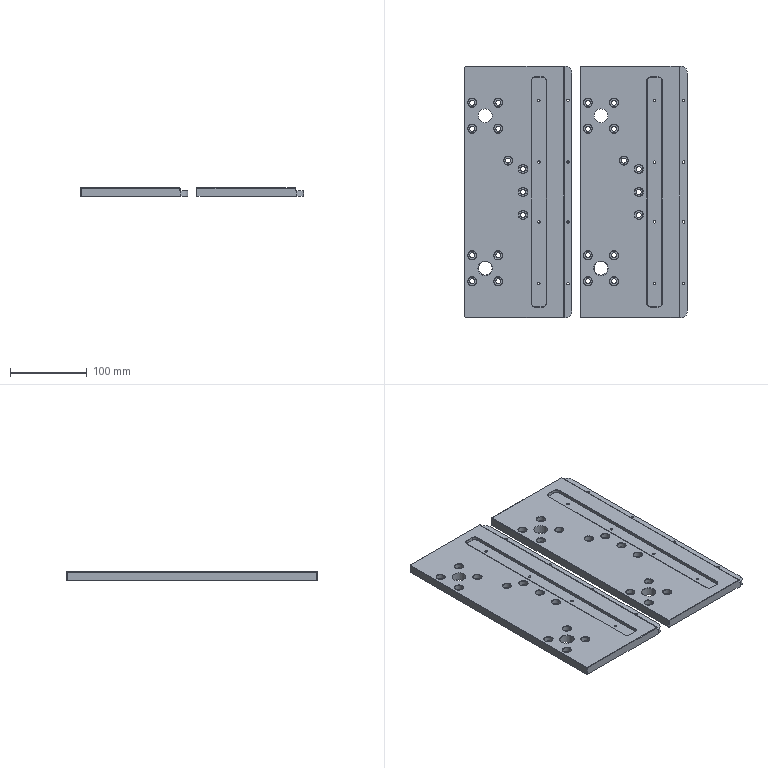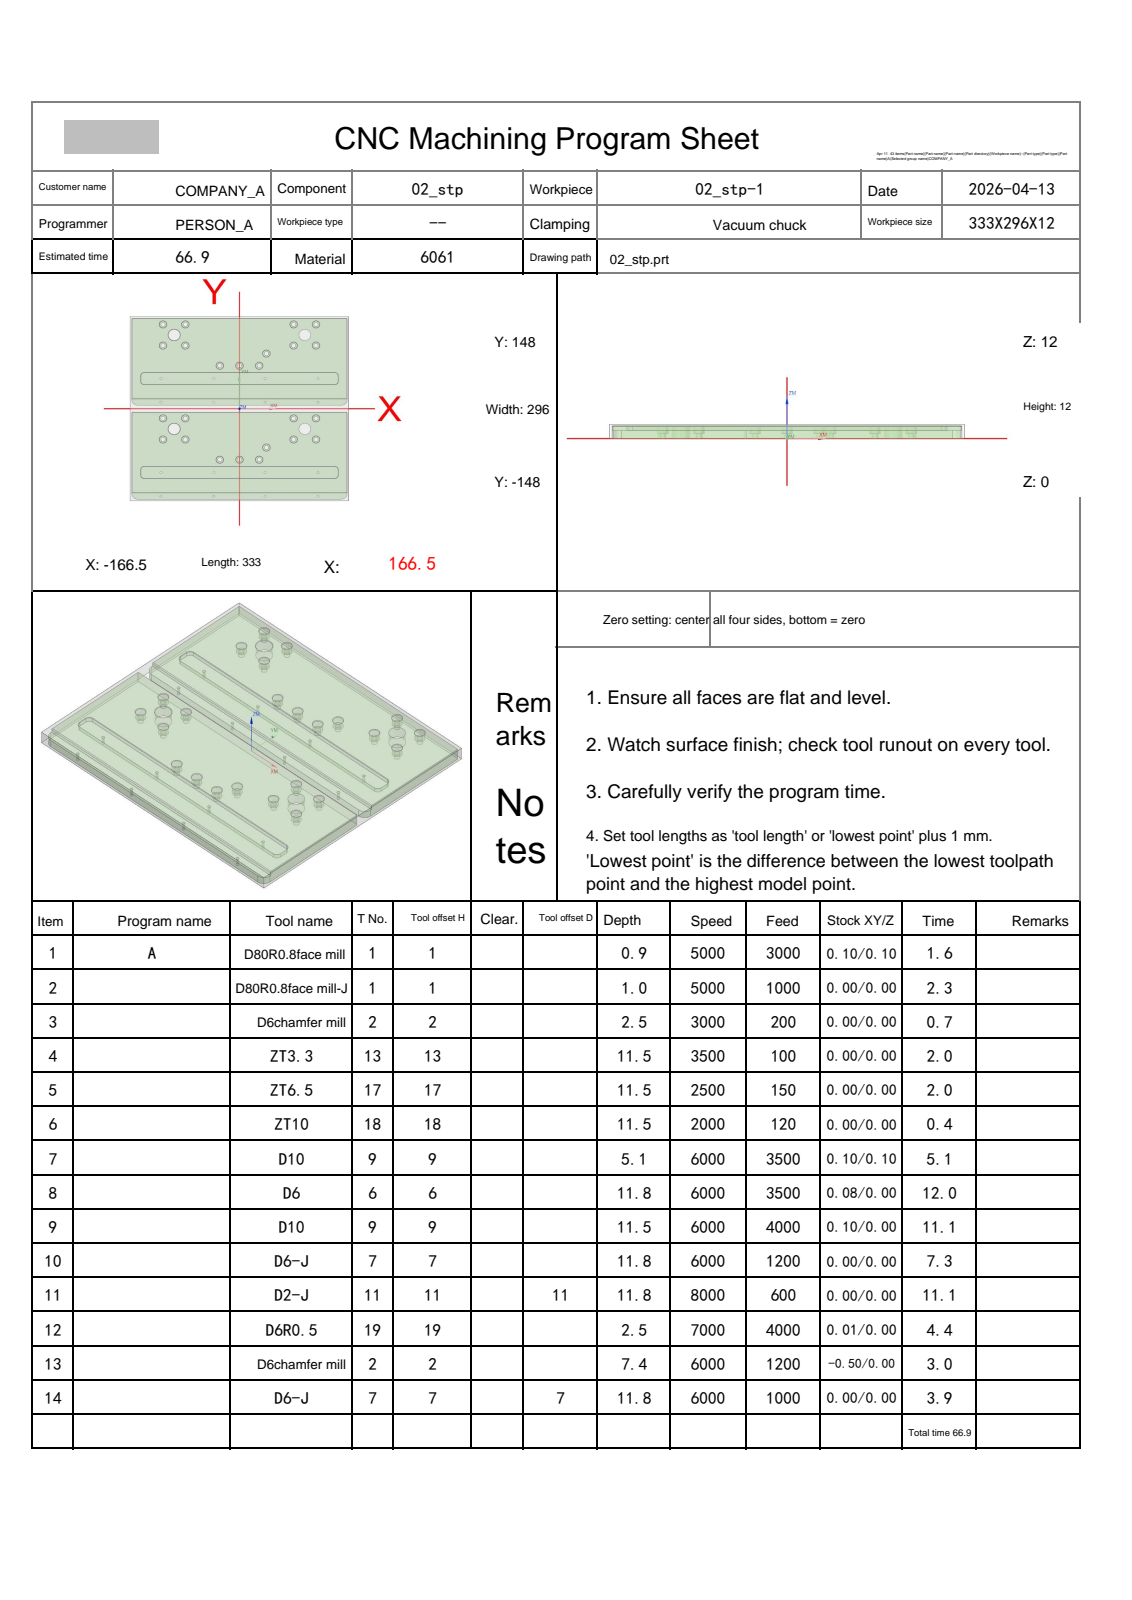NC program | NX | posted by the shop | part box 291 x 328 x 11 mm
Lines 2700 to 3919 of 9762:
N9 T09 M06
(D10  D=10. R=0. H=09 ce=0.10 di=0.00)
G00 G90 G54 X0.0 Y-.4 M03 S6000
G43 H09 Z31.
M08
Z11.5
G01 X163. Z11.415 F4000.
G02 X166.606 Y-1.894 Z11.413 I0.0 J-5.1
G01 X167.606 Y-2.894 Z11.412
G02 X169.1 Y-6.5 Z11.41 I-3.606 J-3.606
G01 Y-136.5 Z11.342
G02 X155. Y-150.6 Z11.331 I-14.1 J0.0
G01 X-155. Z11.169
G02 X-169.1 Y-136.5 Z11.158 I0.0 J14.1
G01 Y-6.5 Z11.09
G02 X-167.606 Y-2.894 Z11.088 I5.1 J0.0
G01 X-166.606 Y-1.894 Z11.087
G02 X-163. Y-.4 Z11.085 I3.606 J-3.606
G01 X163. Z10.915
G02 X166.606 Y-1.894 Z10.913 I0.0 J-5.1
G01 X167.606 Y-2.894 Z10.912
G02 X169.1 Y-6.5 Z10.91 I-3.606 J-3.606
G01 Y-136.5 Z10.842
G02 X155. Y-150.6 Z10.831 I-14.1 J0.0
G01 X-155. Z10.669
G02 X-169.1 Y-136.5 Z10.658 I0.0 J14.1
G01 Y-6.5 Z10.59
G02 X-167.606 Y-2.894 Z10.588 I5.1 J0.0
G01 X-166.606 Y-1.894 Z10.587
G02 X-163. Y-.4 Z10.585 I3.606 J-3.606
G01 X163. Z10.415
G02 X166.606 Y-1.894 Z10.413 I0.0 J-5.1
G01 X167.606 Y-2.894 Z10.412
G02 X169.1 Y-6.5 Z10.41 I-3.606 J-3.606
G01 Y-136.5 Z10.342
G02 X155. Y-150.6 Z10.331 I-14.1 J0.0
G01 X-155. Z10.169
G02 X-169.1 Y-136.5 Z10.158 I0.0 J14.1
G01 Y-6.5 Z10.09
G02 X-167.606 Y-2.894 Z10.088 I5.1 J0.0
G01 X-166.606 Y-1.894 Z10.087
G02 X-163. Y-.4 Z10.085 I3.606 J-3.606
G01 X163. Z9.915
G02 X166.606 Y-1.894 Z9.913 I0.0 J-5.1
G01 X167.606 Y-2.894 Z9.912
G02 X169.1 Y-6.5 Z9.91 I-3.606 J-3.606
G01 Y-136.5 Z9.842
G02 X155. Y-150.6 Z9.831 I-14.1 J0.0
G01 X-155. Z9.669
G02 X-169.1 Y-136.5 Z9.658 I0.0 J14.1
G01 Y-6.5 Z9.59
G02 X-167.606 Y-2.894 Z9.588 I5.1 J0.0
G01 X-166.606 Y-1.894 Z9.587
G02 X-163. Y-.4 Z9.585 I3.606 J-3.606
G01 X163. Z9.415
G02 X166.606 Y-1.894 Z9.413 I0.0 J-5.1
G01 X167.606 Y-2.894 Z9.412
G02 X169.1 Y-6.5 Z9.41 I-3.606 J-3.606
G01 Y-136.5 Z9.342
G02 X155. Y-150.6 Z9.331 I-14.1 J0.0
G01 X-155. Z9.169
G02 X-169.1 Y-136.5 Z9.158 I0.0 J14.1
G01 Y-6.5 Z9.09
G02 X-167.606 Y-2.894 Z9.088 I5.1 J0.0
G01 X-166.606 Y-1.894 Z9.087
G02 X-163. Y-.4 Z9.085 I3.606 J-3.606
G01 X163. Z8.915
G02 X166.606 Y-1.894 Z8.913 I0.0 J-5.1
G01 X167.606 Y-2.894 Z8.912
G02 X169.1 Y-6.5 Z8.91 I-3.606 J-3.606
G01 Y-136.5 Z8.842
G02 X155. Y-150.6 Z8.831 I-14.1 J0.0
G01 X-155. Z8.669
G02 X-169.1 Y-136.5 Z8.658 I0.0 J14.1
G01 Y-6.5 Z8.59
G02 X-167.606 Y-2.894 Z8.588 I5.1 J0.0
G01 X-166.606 Y-1.894 Z8.587
G02 X-163. Y-.4 Z8.585 I3.606 J-3.606
G01 X163. Z8.415
G02 X166.606 Y-1.894 Z8.413 I0.0 J-5.1
G01 X167.606 Y-2.894 Z8.412
G02 X169.1 Y-6.5 Z8.41 I-3.606 J-3.606
G01 Y-136.5 Z8.342
G02 X155. Y-150.6 Z8.331 I-14.1 J0.0
G01 X-155. Z8.169
G02 X-169.1 Y-136.5 Z8.158 I0.0 J14.1
G01 Y-6.5 Z8.09
G02 X-167.606 Y-2.894 Z8.088 I5.1 J0.0
G01 X-166.606 Y-1.894 Z8.087
G02 X-163. Y-.4 Z8.085 I3.606 J-3.606
G01 X163. Z7.915
G02 X166.606 Y-1.894 Z7.913 I0.0 J-5.1
G01 X167.606 Y-2.894 Z7.912
G02 X169.1 Y-6.5 Z7.91 I-3.606 J-3.606
G01 Y-136.5 Z7.842
G02 X155. Y-150.6 Z7.831 I-14.1 J0.0
G01 X-155. Z7.669
G02 X-169.1 Y-136.5 Z7.658 I0.0 J14.1
G01 Y-6.5 Z7.59
G02 X-167.606 Y-2.894 Z7.588 I5.1 J0.0
G01 X-166.606 Y-1.894 Z7.587
G02 X-163. Y-.4 Z7.585 I3.606 J-3.606
G01 X163. Z7.415
G02 X166.606 Y-1.894 Z7.413 I0.0 J-5.1
G01 X167.606 Y-2.894 Z7.412
G02 X169.1 Y-6.5 Z7.41 I-3.606 J-3.606
G01 Y-136.5 Z7.342
G02 X155. Y-150.6 Z7.331 I-14.1 J0.0
G01 X-155. Z7.169
G02 X-169.1 Y-136.5 Z7.158 I0.0 J14.1
G01 Y-6.5 Z7.09
G02 X-167.606 Y-2.894 Z7.088 I5.1 J0.0
G01 X-166.606 Y-1.894 Z7.087
G02 X-163. Y-.4 Z7.085 I3.606 J-3.606
G01 X163. Z6.915
G02 X166.606 Y-1.894 Z6.913 I0.0 J-5.1
G01 X167.606 Y-2.894 Z6.912
G02 X169.1 Y-6.5 Z6.91 I-3.606 J-3.606
G01 Y-136.5 Z6.842
G02 X155. Y-150.6 Z6.831 I-14.1 J0.0
G01 X-155. Z6.669
G02 X-169.1 Y-136.5 Z6.658 I0.0 J14.1
G01 Y-6.5 Z6.59
G02 X-167.606 Y-2.894 Z6.588 I5.1 J0.0
G01 X-166.606 Y-1.894 Z6.587
G02 X-163. Y-.4 Z6.585 I3.606 J-3.606
G01 X163. Z6.415
G02 X166.606 Y-1.894 Z6.413 I0.0 J-5.1
G01 X167.606 Y-2.894 Z6.412
G02 X169.1 Y-6.5 Z6.41 I-3.606 J-3.606
G01 Y-136.5 Z6.342
G02 X155. Y-150.6 Z6.331 I-14.1 J0.0
G01 X-155. Z6.169
G02 X-169.1 Y-136.5 Z6.158 I0.0 J14.1
G01 Y-6.5 Z6.09
G02 X-167.606 Y-2.894 Z6.088 I5.1 J0.0
G01 X-166.606 Y-1.894 Z6.087
G02 X-163. Y-.4 Z6.085 I3.606 J-3.606
G01 X163. Z5.915
G02 X166.606 Y-1.894 Z5.913 I0.0 J-5.1
G01 X167.606 Y-2.894 Z5.912
G02 X169.1 Y-6.5 Z5.91 I-3.606 J-3.606
G01 Y-136.5 Z5.842
G02 X155. Y-150.6 Z5.831 I-14.1 J0.0
G01 X-155. Z5.669
G02 X-169.1 Y-136.5 Z5.658 I0.0 J14.1
G01 Y-6.5 Z5.59
G02 X-167.606 Y-2.894 Z5.588 I5.1 J0.0
G01 X-166.606 Y-1.894 Z5.587
G02 X-163. Y-.4 Z5.585 I3.606 J-3.606
G01 X163. Z5.415
G02 X166.606 Y-1.894 Z5.413 I0.0 J-5.1
G01 X167.606 Y-2.894 Z5.412
G02 X169.1 Y-6.5 Z5.41 I-3.606 J-3.606
G01 Y-136.5 Z5.342
G02 X155. Y-150.6 Z5.331 I-14.1 J0.0
G01 X-155. Z5.169
G02 X-169.1 Y-136.5 Z5.158 I0.0 J14.1
G01 Y-6.5 Z5.09
G02 X-167.606 Y-2.894 Z5.088 I5.1 J0.0
G01 X-166.606 Y-1.894 Z5.087
G02 X-163. Y-.4 Z5.085 I3.606 J-3.606
G01 X163. Z4.915
G02 X166.606 Y-1.894 Z4.913 I0.0 J-5.1
G01 X167.606 Y-2.894 Z4.912
G02 X169.1 Y-6.5 Z4.91 I-3.606 J-3.606
G01 Y-136.5 Z4.842
G02 X155. Y-150.6 Z4.831 I-14.1 J0.0
G01 X-155. Z4.669
G02 X-169.1 Y-136.5 Z4.658 I0.0 J14.1
G01 Y-6.5 Z4.59
G02 X-167.606 Y-2.894 Z4.588 I5.1 J0.0
G01 X-166.606 Y-1.894 Z4.587
G02 X-163. Y-.4 Z4.585 I3.606 J-3.606
G01 X163. Z4.415
G02 X166.606 Y-1.894 Z4.413 I0.0 J-5.1
G01 X167.606 Y-2.894 Z4.412
G02 X169.1 Y-6.5 Z4.41 I-3.606 J-3.606
G01 Y-136.5 Z4.342
G02 X155. Y-150.6 Z4.331 I-14.1 J0.0
G01 X-155. Z4.169
G02 X-169.1 Y-136.5 Z4.158 I0.0 J14.1
G01 Y-6.5 Z4.09
G02 X-167.606 Y-2.894 Z4.088 I5.1 J0.0
G01 X-166.606 Y-1.894 Z4.087
G02 X-163. Y-.4 Z4.085 I3.606 J-3.606
G01 X163. Z3.915
G02 X166.606 Y-1.894 Z3.913 I0.0 J-5.1
G01 X167.606 Y-2.894 Z3.912
G02 X169.1 Y-6.5 Z3.91 I-3.606 J-3.606
G01 Y-136.5 Z3.842
G02 X155. Y-150.6 Z3.831 I-14.1 J0.0
G01 X-155. Z3.669
G02 X-169.1 Y-136.5 Z3.658 I0.0 J14.1
G01 Y-6.5 Z3.59
G02 X-167.606 Y-2.894 Z3.588 I5.1 J0.0
G01 X-166.606 Y-1.894 Z3.587
G02 X-163. Y-.4 Z3.585 I3.606 J-3.606
G01 X163. Z3.415
G02 X166.606 Y-1.894 Z3.413 I0.0 J-5.1
G01 X167.606 Y-2.894 Z3.412
G02 X169.1 Y-6.5 Z3.41 I-3.606 J-3.606
G01 Y-136.5 Z3.342
G02 X155. Y-150.6 Z3.331 I-14.1 J0.0
G01 X-155. Z3.169
G02 X-169.1 Y-136.5 Z3.158 I0.0 J14.1
G01 Y-6.5 Z3.09
G02 X-167.606 Y-2.894 Z3.088 I5.1 J0.0
G01 X-166.606 Y-1.894 Z3.087
G02 X-163. Y-.4 Z3.085 I3.606 J-3.606
G01 X163. Z2.915
G02 X166.606 Y-1.894 Z2.913 I0.0 J-5.1
G01 X167.606 Y-2.894 Z2.912
G02 X169.1 Y-6.5 Z2.91 I-3.606 J-3.606
G01 Y-136.5 Z2.842
G02 X155. Y-150.6 Z2.831 I-14.1 J0.0
G01 X-155. Z2.669
G02 X-169.1 Y-136.5 Z2.658 I0.0 J14.1
G01 Y-6.5 Z2.59
G02 X-167.606 Y-2.894 Z2.588 I5.1 J0.0
G01 X-166.606 Y-1.894 Z2.587
G02 X-163. Y-.4 Z2.585 I3.606 J-3.606
G01 X163. Z2.415
G02 X166.606 Y-1.894 Z2.413 I0.0 J-5.1
G01 X167.606 Y-2.894 Z2.412
G02 X169.1 Y-6.5 Z2.41 I-3.606 J-3.606
G01 Y-136.5 Z2.342
G02 X155. Y-150.6 Z2.331 I-14.1 J0.0
G01 X-155. Z2.169
G02 X-169.1 Y-136.5 Z2.158 I0.0 J14.1
G01 Y-6.5 Z2.09
G02 X-167.606 Y-2.894 Z2.088 I5.1 J0.0
G01 X-166.606 Y-1.894 Z2.087
G02 X-163. Y-.4 Z2.085 I3.606 J-3.606
G01 X163. Z1.915
G02 X166.606 Y-1.894 Z1.913 I0.0 J-5.1
G01 X167.606 Y-2.894 Z1.912
G02 X169.1 Y-6.5 Z1.91 I-3.606 J-3.606
G01 Y-136.5 Z1.842
G02 X155. Y-150.6 Z1.831 I-14.1 J0.0
G01 X-155. Z1.669
G02 X-169.1 Y-136.5 Z1.658 I0.0 J14.1
G01 Y-6.5 Z1.59
G02 X-167.606 Y-2.894 Z1.588 I5.1 J0.0
G01 X-166.606 Y-1.894 Z1.587
G02 X-163. Y-.4 Z1.585 I3.606 J-3.606
G01 X163. Z1.415
G02 X166.606 Y-1.894 Z1.413 I0.0 J-5.1
G01 X167.606 Y-2.894 Z1.412
G02 X169.1 Y-6.5 Z1.41 I-3.606 J-3.606
G01 Y-136.5 Z1.342
G02 X155. Y-150.6 Z1.331 I-14.1 J0.0
G01 X-155. Z1.169
G02 X-169.1 Y-136.5 Z1.158 I0.0 J14.1
G01 Y-6.5 Z1.09
G02 X-167.606 Y-2.894 Z1.088 I5.1 J0.0
G01 X-166.606 Y-1.894 Z1.087
G02 X-163. Y-.4 Z1.085 I3.606 J-3.606
G01 X163. Z.915
G02 X166.606 Y-1.894 Z.913 I0.0 J-5.1
G01 X167.606 Y-2.894 Z.912
G02 X169.1 Y-6.5 Z.91 I-3.606 J-3.606
G01 Y-136.5 Z.842
G02 X155. Y-150.6 Z.831 I-14.1 J0.0
G01 X-155. Z.669
G02 X-169.1 Y-136.5 Z.658 I0.0 J14.1
G01 Y-6.5 Z.59
G02 X-167.606 Y-2.894 Z.588 I5.1 J0.0
G01 X-166.606 Y-1.894 Z.587
G02 X-163. Y-.4 Z.585 I3.606 J-3.606
G01 X0.0 Z.5
X163.
G02 X166.606 Y-1.894 I0.0 J-5.1
G01 X167.606 Y-2.894
G02 X169.1 Y-6.5 I-3.606 J-3.606
G01 Y-136.5
G02 X155. Y-150.6 I-14.1 J0.0
G01 X-155.
G02 X-169.1 Y-136.5 I0.0 J14.1
G01 Y-6.5
G02 X-167.606 Y-2.894 I5.1 J0.0
G01 X-166.606 Y-1.894
G02 X-163. Y-.4 I3.606 J-3.606
G01 X0.0
X.5
Z1.5
G00 Z31.
X0.0 Y150.6
Z11.5
G01 X163. Z11.415
G02 X166.606 Y149.106 Z11.413 I0.0 J-5.1
G01 X167.606 Y148.106 Z11.412
G02 X169.1 Y144.5 Z11.41 I-3.606 J-3.606
G01 Y14.5 Z11.342
G02 X155. Y.4 Z11.331 I-14.1 J0.0
G01 X-155. Z11.169
G02 X-169.1 Y14.5 Z11.158 I0.0 J14.1
G01 Y144.5 Z11.09
G02 X-167.606 Y148.106 Z11.088 I5.1 J0.0
G01 X-166.606 Y149.106 Z11.087
G02 X-163. Y150.6 Z11.085 I3.606 J-3.606
G01 X163. Z10.915
G02 X166.606 Y149.106 Z10.913 I0.0 J-5.1
G01 X167.606 Y148.106 Z10.912
G02 X169.1 Y144.5 Z10.91 I-3.606 J-3.606
G01 Y14.5 Z10.842
G02 X155. Y.4 Z10.831 I-14.1 J0.0
G01 X-155. Z10.669
G02 X-169.1 Y14.5 Z10.658 I0.0 J14.1
G01 Y144.5 Z10.59
G02 X-167.606 Y148.106 Z10.588 I5.1 J0.0
G01 X-166.606 Y149.106 Z10.587
G02 X-163. Y150.6 Z10.585 I3.606 J-3.606
G01 X163. Z10.415
G02 X166.606 Y149.106 Z10.413 I0.0 J-5.1
G01 X167.606 Y148.106 Z10.412
G02 X169.1 Y144.5 Z10.41 I-3.606 J-3.606
G01 Y14.5 Z10.342
G02 X155. Y.4 Z10.331 I-14.1 J0.0
G01 X-155. Z10.169
G02 X-169.1 Y14.5 Z10.158 I0.0 J14.1
G01 Y144.5 Z10.09
G02 X-167.606 Y148.106 Z10.088 I5.1 J0.0
G01 X-166.606 Y149.106 Z10.087
G02 X-163. Y150.6 Z10.085 I3.606 J-3.606
G01 X163. Z9.915
G02 X166.606 Y149.106 Z9.913 I0.0 J-5.1
G01 X167.606 Y148.106 Z9.912
G02 X169.1 Y144.5 Z9.91 I-3.606 J-3.606
G01 Y14.5 Z9.842
G02 X155. Y.4 Z9.831 I-14.1 J0.0
G01 X-155. Z9.669
G02 X-169.1 Y14.5 Z9.658 I0.0 J14.1
G01 Y144.5 Z9.59
G02 X-167.606 Y148.106 Z9.588 I5.1 J0.0
G01 X-166.606 Y149.106 Z9.587
G02 X-163. Y150.6 Z9.585 I3.606 J-3.606
G01 X163. Z9.415
G02 X166.606 Y149.106 Z9.413 I0.0 J-5.1
G01 X167.606 Y148.106 Z9.412
G02 X169.1 Y144.5 Z9.41 I-3.606 J-3.606
G01 Y14.5 Z9.342
G02 X155. Y.4 Z9.331 I-14.1 J0.0
G01 X-155. Z9.169
G02 X-169.1 Y14.5 Z9.158 I0.0 J14.1
G01 Y144.5 Z9.09
G02 X-167.606 Y148.106 Z9.088 I5.1 J0.0
G01 X-166.606 Y149.106 Z9.087
G02 X-163. Y150.6 Z9.085 I3.606 J-3.606
G01 X163. Z8.915
G02 X166.606 Y149.106 Z8.913 I0.0 J-5.1
G01 X167.606 Y148.106 Z8.912
G02 X169.1 Y144.5 Z8.91 I-3.606 J-3.606
G01 Y14.5 Z8.842
G02 X155. Y.4 Z8.831 I-14.1 J0.0
G01 X-155. Z8.669
G02 X-169.1 Y14.5 Z8.658 I0.0 J14.1
G01 Y144.5 Z8.59
G02 X-167.606 Y148.106 Z8.588 I5.1 J0.0
G01 X-166.606 Y149.106 Z8.587
G02 X-163. Y150.6 Z8.585 I3.606 J-3.606
G01 X163. Z8.415
G02 X166.606 Y149.106 Z8.413 I0.0 J-5.1
G01 X167.606 Y148.106 Z8.412
G02 X169.1 Y144.5 Z8.41 I-3.606 J-3.606
G01 Y14.5 Z8.342
G02 X155. Y.4 Z8.331 I-14.1 J0.0
G01 X-155. Z8.169
G02 X-169.1 Y14.5 Z8.158 I0.0 J14.1
G01 Y144.5 Z8.09
G02 X-167.606 Y148.106 Z8.088 I5.1 J0.0
G01 X-166.606 Y149.106 Z8.087
G02 X-163. Y150.6 Z8.085 I3.606 J-3.606
G01 X163. Z7.915
G02 X166.606 Y149.106 Z7.913 I0.0 J-5.1
G01 X167.606 Y148.106 Z7.912
G02 X169.1 Y144.5 Z7.91 I-3.606 J-3.606
G01 Y14.5 Z7.842
G02 X155. Y.4 Z7.831 I-14.1 J0.0
G01 X-155. Z7.669
G02 X-169.1 Y14.5 Z7.658 I0.0 J14.1
G01 Y144.5 Z7.59
G02 X-167.606 Y148.106 Z7.588 I5.1 J0.0
G01 X-166.606 Y149.106 Z7.587
G02 X-163. Y150.6 Z7.585 I3.606 J-3.606
G01 X163. Z7.415
G02 X166.606 Y149.106 Z7.413 I0.0 J-5.1
G01 X167.606 Y148.106 Z7.412
G02 X169.1 Y144.5 Z7.41 I-3.606 J-3.606
G01 Y14.5 Z7.342
G02 X155. Y.4 Z7.331 I-14.1 J0.0
G01 X-155. Z7.169
G02 X-169.1 Y14.5 Z7.158 I0.0 J14.1
G01 Y144.5 Z7.09
G02 X-167.606 Y148.106 Z7.088 I5.1 J0.0
G01 X-166.606 Y149.106 Z7.087
G02 X-163. Y150.6 Z7.085 I3.606 J-3.606
G01 X163. Z6.915
G02 X166.606 Y149.106 Z6.913 I0.0 J-5.1
G01 X167.606 Y148.106 Z6.912
G02 X169.1 Y144.5 Z6.91 I-3.606 J-3.606
G01 Y14.5 Z6.842
G02 X155. Y.4 Z6.831 I-14.1 J0.0
G01 X-155. Z6.669
G02 X-169.1 Y14.5 Z6.658 I0.0 J14.1
G01 Y144.5 Z6.59
G02 X-167.606 Y148.106 Z6.588 I5.1 J0.0
G01 X-166.606 Y149.106 Z6.587
G02 X-163. Y150.6 Z6.585 I3.606 J-3.606
G01 X163. Z6.415
G02 X166.606 Y149.106 Z6.413 I0.0 J-5.1
G01 X167.606 Y148.106 Z6.412
G02 X169.1 Y144.5 Z6.41 I-3.606 J-3.606
G01 Y14.5 Z6.342
G02 X155. Y.4 Z6.331 I-14.1 J0.0
G01 X-155. Z6.169
G02 X-169.1 Y14.5 Z6.158 I0.0 J14.1
G01 Y144.5 Z6.09
G02 X-167.606 Y148.106 Z6.088 I5.1 J0.0
G01 X-166.606 Y149.106 Z6.087
G02 X-163. Y150.6 Z6.085 I3.606 J-3.606
G01 X163. Z5.915
G02 X166.606 Y149.106 Z5.913 I0.0 J-5.1
G01 X167.606 Y148.106 Z5.912
G02 X169.1 Y144.5 Z5.91 I-3.606 J-3.606
G01 Y14.5 Z5.842
G02 X155. Y.4 Z5.831 I-14.1 J0.0
G01 X-155. Z5.669
G02 X-169.1 Y14.5 Z5.658 I0.0 J14.1
G01 Y144.5 Z5.59
G02 X-167.606 Y148.106 Z5.588 I5.1 J0.0
G01 X-166.606 Y149.106 Z5.587
G02 X-163. Y150.6 Z5.585 I3.606 J-3.606
G01 X163. Z5.415
G02 X166.606 Y149.106 Z5.413 I0.0 J-5.1
G01 X167.606 Y148.106 Z5.412
G02 X169.1 Y144.5 Z5.41 I-3.606 J-3.606
G01 Y14.5 Z5.342
G02 X155. Y.4 Z5.331 I-14.1 J0.0
G01 X-155. Z5.169
G02 X-169.1 Y14.5 Z5.158 I0.0 J14.1
G01 Y144.5 Z5.09
G02 X-167.606 Y148.106 Z5.088 I5.1 J0.0
G01 X-166.606 Y149.106 Z5.087
G02 X-163. Y150.6 Z5.085 I3.606 J-3.606
G01 X163. Z4.915
G02 X166.606 Y149.106 Z4.913 I0.0 J-5.1
G01 X167.606 Y148.106 Z4.912
G02 X169.1 Y144.5 Z4.91 I-3.606 J-3.606
G01 Y14.5 Z4.842
G02 X155. Y.4 Z4.831 I-14.1 J0.0
G01 X-155. Z4.669
G02 X-169.1 Y14.5 Z4.658 I0.0 J14.1
G01 Y144.5 Z4.59
G02 X-167.606 Y148.106 Z4.588 I5.1 J0.0
G01 X-166.606 Y149.106 Z4.587
G02 X-163. Y150.6 Z4.585 I3.606 J-3.606
G01 X163. Z4.415
G02 X166.606 Y149.106 Z4.413 I0.0 J-5.1
G01 X167.606 Y148.106 Z4.412
G02 X169.1 Y144.5 Z4.41 I-3.606 J-3.606
G01 Y14.5 Z4.342
G02 X155. Y.4 Z4.331 I-14.1 J0.0
G01 X-155. Z4.169
G02 X-169.1 Y14.5 Z4.158 I0.0 J14.1
G01 Y144.5 Z4.09
G02 X-167.606 Y148.106 Z4.088 I5.1 J0.0
G01 X-166.606 Y149.106 Z4.087
G02 X-163. Y150.6 Z4.085 I3.606 J-3.606
G01 X163. Z3.915
G02 X166.606 Y149.106 Z3.913 I0.0 J-5.1
G01 X167.606 Y148.106 Z3.912
G02 X169.1 Y144.5 Z3.91 I-3.606 J-3.606
G01 Y14.5 Z3.842
G02 X155. Y.4 Z3.831 I-14.1 J0.0
G01 X-155. Z3.669
G02 X-169.1 Y14.5 Z3.658 I0.0 J14.1
G01 Y144.5 Z3.59
G02 X-167.606 Y148.106 Z3.588 I5.1 J0.0
G01 X-166.606 Y149.106 Z3.587
G02 X-163. Y150.6 Z3.585 I3.606 J-3.606
G01 X163. Z3.415
G02 X166.606 Y149.106 Z3.413 I0.0 J-5.1
G01 X167.606 Y148.106 Z3.412
G02 X169.1 Y144.5 Z3.41 I-3.606 J-3.606
G01 Y14.5 Z3.342
G02 X155. Y.4 Z3.331 I-14.1 J0.0
G01 X-155. Z3.169
G02 X-169.1 Y14.5 Z3.158 I0.0 J14.1
G01 Y144.5 Z3.09
G02 X-167.606 Y148.106 Z3.088 I5.1 J0.0
G01 X-166.606 Y149.106 Z3.087
G02 X-163. Y150.6 Z3.085 I3.606 J-3.606
G01 X163. Z2.915
G02 X166.606 Y149.106 Z2.913 I0.0 J-5.1
G01 X167.606 Y148.106 Z2.912
G02 X169.1 Y144.5 Z2.91 I-3.606 J-3.606
G01 Y14.5 Z2.842
G02 X155. Y.4 Z2.831 I-14.1 J0.0
G01 X-155. Z2.669
G02 X-169.1 Y14.5 Z2.658 I0.0 J14.1
G01 Y144.5 Z2.59
G02 X-167.606 Y148.106 Z2.588 I5.1 J0.0
G01 X-166.606 Y149.106 Z2.587
G02 X-163. Y150.6 Z2.585 I3.606 J-3.606
G01 X163. Z2.415
G02 X166.606 Y149.106 Z2.413 I0.0 J-5.1
G01 X167.606 Y148.106 Z2.412
G02 X169.1 Y144.5 Z2.41 I-3.606 J-3.606
G01 Y14.5 Z2.342
G02 X155. Y.4 Z2.331 I-14.1 J0.0
G01 X-155. Z2.169
G02 X-169.1 Y14.5 Z2.158 I0.0 J14.1
G01 Y144.5 Z2.09
G02 X-167.606 Y148.106 Z2.088 I5.1 J0.0
G01 X-166.606 Y149.106 Z2.087
G02 X-163. Y150.6 Z2.085 I3.606 J-3.606
G01 X163. Z1.915
G02 X166.606 Y149.106 Z1.913 I0.0 J-5.1
G01 X167.606 Y148.106 Z1.912
G02 X169.1 Y144.5 Z1.91 I-3.606 J-3.606
G01 Y14.5 Z1.842
G02 X155. Y.4 Z1.831 I-14.1 J0.0
G01 X-155. Z1.669
G02 X-169.1 Y14.5 Z1.658 I0.0 J14.1
G01 Y144.5 Z1.59
G02 X-167.606 Y148.106 Z1.588 I5.1 J0.0
G01 X-166.606 Y149.106 Z1.587
G02 X-163. Y150.6 Z1.585 I3.606 J-3.606
G01 X163. Z1.415
G02 X166.606 Y149.106 Z1.413 I0.0 J-5.1
G01 X167.606 Y148.106 Z1.412
G02 X169.1 Y144.5 Z1.41 I-3.606 J-3.606
G01 Y14.5 Z1.342
G02 X155. Y.4 Z1.331 I-14.1 J0.0
G01 X-155. Z1.169
G02 X-169.1 Y14.5 Z1.158 I0.0 J14.1
G01 Y144.5 Z1.09
G02 X-167.606 Y148.106 Z1.088 I5.1 J0.0
G01 X-166.606 Y149.106 Z1.087
G02 X-163. Y150.6 Z1.085 I3.606 J-3.606
G01 X163. Z.915
G02 X166.606 Y149.106 Z.913 I0.0 J-5.1
G01 X167.606 Y148.106 Z.912
G02 X169.1 Y144.5 Z.91 I-3.606 J-3.606
G01 Y14.5 Z.842
G02 X155. Y.4 Z.831 I-14.1 J0.0
G01 X-155. Z.669
G02 X-169.1 Y14.5 Z.658 I0.0 J14.1
G01 Y144.5 Z.59
G02 X-167.606 Y148.106 Z.588 I5.1 J0.0
G01 X-166.606 Y149.106 Z.587
G02 X-163. Y150.6 Z.585 I3.606 J-3.606
G01 X0.0 Z.5
X163.
G02 X166.606 Y149.106 I0.0 J-5.1
G01 X167.606 Y148.106
G02 X169.1 Y144.5 I-3.606 J-3.606
G01 Y14.5
G02 X155. Y.4 I-14.1 J0.0
G01 X-155.
G02 X-169.1 Y14.5 I0.0 J14.1
G01 Y144.5
G02 X-167.606 Y148.106 I5.1 J0.0
G01 X-166.606 Y149.106
G02 X-163. Y150.6 I3.606 J-3.606
G01 X0.0
X.5
Z1.5
G00 Z31.
G91 G28 Z0.0
M05
M09
G91 G28 Z0.0
M01
N10 T07 M06
(D6-J  D=6. R=0. H=07 ce=0.30 di=0.00)
G00 G90 G54 X161.108 Y.8 M03 S6000
G43 H07 Z31.
M08
Z7.5
G01 Z7. F1200.
X159.898 Y2.242
X158.562 Y5.585
G02 X155. Y4.9 I-3.562 J8.915
G01 X-155.
G02 X-164.32 Y12.2 I0.0 J9.6
G01 X164.32
G02 X158.562 Y5.585 I-9.32 J2.3
G01 X157.56 Y8.093
G02 X155. Y7.6 I-2.56 J6.407
G01 X-155.
G02 X-159.755 Y9.5 I0.0 J6.9
G01 X159.755
G02 X157.56 Y8.093 I-4.755 J5.
X157.09 Y7.924 I-2.56 J6.407
G01 X158.18 Y4.493
X161.108 Y.8
Z7.5
G00 Z31.
X0.0 Y-151.5
Z7.5
G01 Z7.
Y-146.1
X-155.
G02 X-164.32 Y-138.8 I0.0 J9.6
G01 X164.32
G02 X155. Y-146.1 I-9.32 J2.3
G01 X0.0
Y-143.4
X-155.
G02 X-159.755 Y-141.5 I0.0 J6.9
G01 X159.755
G02 X155. Y-143.4 I-4.755 J5.
G01 X0.0
X-.5
Y-151.5
Z7.5
G00 Z31.
G00 G90 X42.954 Y-108.75 M03 S6000
Z31.
Z8.3
G01 X0.0 Z6.8 F1200.
X-145.
G02 X-146.75 Y-107. I0.0 J1.75
G01 Y-98.
G02 X-145. Y-96.25 I1.75 J0.0
G01 X145.
G02 X146.75 Y-98. I0.0 J-1.75
G01 Y-107.
G02 X145. Y-108.75 I-1.75 J0.0
G01 X0.0
Y-104.55
X-142.55
Y-100.45
X142.55
Y-104.55
X0.0
X-.5
Y-108.15
Z7.3
G00 Z31.
X-42.954 Y54.75
Z8.3
G01 X0.0 Z6.8
X145.
G02 X146.75 Y53. I0.0 J-1.75
G01 Y44.
G02 X145. Y42.25 I-1.75 J0.0
G01 X-145.
G02 X-146.75 Y44. I0.0 J1.75
G01 Y53.
G02 X-145. Y54.75 I1.75 J0.0
G01 X0.0
Y50.55
X142.55
Y46.45
X-142.55
Y50.55
X0.0
X.5
Y54.15
Z7.3
G00 Z31.
G00 G90 X168.093 Y14.875 M03 S6000
Z31.
Z7.505
G01 Z7.005 F1200.
G41 D07
X168. Y14.911
G03 X167.636 Y14.98 I-.364 J-.932
X166.929 Y14.687 I0.0 J-1.
G01 X164.743 Y12.5
X-164.743
X-166.929 Y14.687
G03 X-167.636 Y14.98 I-.707 J-.707
X-168. Y14.911 I0.0 J-1.
G01 G40 X-168.093 Y14.875
Z7.505
G00 Z31.
X168.093 Y-136.125
Z7.505
G01 Z7.005
G41 D07
X168. Y-136.089
G03 X167.636 Y-136.02 I-.364 J-.932
X166.929 Y-136.313 I0.0 J-1.
G01 X164.743 Y-138.5
X-164.743
X-166.929 Y-136.313
G03 X-167.636 Y-136.02 I-.707 J-.707
X-168. Y-136.089 I0.0 J-1.
G01 G40 X-168.093 Y-136.125
Z7.505
G00 Z31.
G00 G90 X1. Y53.95 M03 S6000
Z31.
Z7.305
G01 Z6.805 F1200.
G41 D07
Y54.05
G03 X0.0 Y55.05 I-1. J0.0
G01 X-145.
G03 X-147.05 Y53. I0.0 J-2.05
G01 Y44.
G03 X-145. Y41.95 I2.05 J0.0
G01 X145.
G03 X147.05 Y44. I0.0 J2.05
G01 Y53.
G03 X145. Y55.05 I-2.05 J0.0
G01 X0.0
X-.5
G03 X-1.5 Y54.05 I0.0 J-1.
G01 G40 Y53.95
Z7.305
G00 Z31.
X-1. Y-107.95
Z7.305
G01 Z6.805
G41 D07
Y-108.05
G03 X0.0 Y-109.05 I1. J0.0
G01 X145.
G03 X147.05 Y-107. I0.0 J2.05
G01 Y-98.
G03 X145. Y-95.95 I-2.05 J0.0
G01 X-145.
G03 X-147.05 Y-98. I0.0 J-2.05
G01 Y-107.
G03 X-145. Y-109.05 I2.05 J0.0
G01 X0.0
X.5
G03 X1.5 Y-108.05 I0.0 J1.
G01 G40 Y-107.95
Z7.305
G00 Z31.
G00 G90 X41. Y-62.4 M03 S6000
Z31.
Z4.5
G41 D07
G01 X40.638 Y-64.468 F800.
X40.632 Y-64.532
G03 X41. Y-64.9 I.368 J0.0
X43.5 Y-62.4 I0.0 J2.5
X41. Y-59.9 I-2.5 J0.0
X38.5 Y-62.4 I0.0 J-2.5
X41. Y-64.9 I2.5 J0.0
X41.497 Y-64.85 I0.0 J2.5
X41.792 Y-64.49 I-.073 J.361
G01 X41.766 Y-64.355
G40 X41. Y-62.4
G00 Z31.
X82.5 Y-15.5
Z4.5
G41 D07
G01 X82.138 Y-17.568
X82.132 Y-17.632
G03 X82.5 Y-18. I.368 J0.0
X85. Y-15.5 I0.0 J2.5
X82.5 Y-13. I-2.5 J0.0
X80. Y-15.5 I0.0 J-2.5
X82.5 Y-18. I2.5 J0.0
X82.997 Y-17.95 I0.0 J2.5
X83.292 Y-17.59 I-.073 J.361
G01 X83.266 Y-17.455
G40 X82.5 Y-15.5
G00 Z31.
X116.5
Z4.5
G41 D07
G01 X116.138 Y-17.568
X116.132 Y-17.632
G03 X116.5 Y-18. I.368 J0.0
X119. Y-15.5 I0.0 J2.5
X116.5 Y-13. I-2.5 J0.0
X114. Y-15.5 I0.0 J-2.5
X116.5 Y-18. I2.5 J0.0
X116.997 Y-17.95 I0.0 J2.5
X117.292 Y-17.59 I-.073 J.361
G01 X117.266 Y-17.455
G40 X116.5 Y-15.5
G00 Z31.
Y-49.5
Z4.5
G41 D07
G01 X116.138 Y-51.568
X116.132 Y-51.632
G03 X116.5 Y-52. I.368 J0.0
X119. Y-49.5 I0.0 J2.5
X116.5 Y-47. I-2.5 J0.0
X114. Y-49.5 I0.0 J-2.5
X116.5 Y-52. I2.5 J0.0
X116.997 Y-51.95 I0.0 J2.5
X117.292 Y-51.59 I-.073 J.361
G01 X117.266 Y-51.455
G40 X116.5 Y-49.5
G00 Z31.
X82.5
Z4.5
G41 D07
G01 X82.138 Y-51.568
X82.132 Y-51.632
G03 X82.5 Y-52. I.368 J0.0
X85. Y-49.5 I0.0 J2.5
X82.5 Y-47. I-2.5 J0.0
X80. Y-49.5 I0.0 J-2.5
X82.5 Y-52. I2.5 J0.0
X82.997 Y-51.95 I0.0 J2.5
X83.292 Y-51.59 I-.073 J.361
G01 X83.266 Y-51.455
G40 X82.5 Y-49.5
G00 Z31.
X30.05 Y-81.9
Z4.5
G41 D07
G01 X29.688 Y-83.968
X29.682 Y-84.032
G03 X30.05 Y-84.4 I.368 J0.0
X32.55 Y-81.9 I0.0 J2.5
X30.05 Y-79.4 I-2.5 J0.0
X27.55 Y-81.9 I0.0 J-2.5
X30.05 Y-84.4 I2.5 J0.0
X30.547 Y-84.35 I0.0 J2.5
X30.842 Y-83.99 I-.073 J.361
G01 X30.816 Y-83.855
G40 X30.05 Y-81.9
G00 Z31.
X.05
Z4.5
G41 D07
G01 X-.312 Y-83.968
X-.318 Y-84.032
G03 X.05 Y-84.4 I.368 J0.0
X2.55 Y-81.9 I0.0 J2.5
X.05 Y-79.4 I-2.5 J0.0
X-2.45 Y-81.9 I0.0 J-2.5
X.05 Y-84.4 I2.5 J0.0
X.547 Y-84.35 I0.0 J2.5
X.842 Y-83.99 I-.073 J.361
G01 X.816 Y-83.855
G40 X.05 Y-81.9
G00 Z31.
X-29.95
Z4.5
G41 D07
G01 X-30.312 Y-83.968
X-30.318 Y-84.032
G03 X-29.95 Y-84.4 I.368 J0.0
X-27.45 Y-81.9 I0.0 J2.5
X-29.95 Y-79.4 I-2.5 J0.0
X-32.45 Y-81.9 I0.0 J-2.5
X-29.95 Y-84.4 I2.5 J0.0
X-29.453 Y-84.35 I0.0 J2.5
X-29.158 Y-83.99 I-.073 J.361
G01 X-29.184 Y-83.855
G40 X-29.95 Y-81.9
G00 Z31.
X-82.5 Y-49.5
Z4.5
G41 D07
G01 X-82.862 Y-51.568
X-82.868 Y-51.632
G03 X-82.5 Y-52. I.368 J0.0
X-80. Y-49.5 I0.0 J2.5
X-82.5 Y-47. I-2.5 J0.0
X-85. Y-49.5 I0.0 J-2.5
X-82.5 Y-52. I2.5 J0.0
X-82.003 Y-51.95 I0.0 J2.5
X-81.708 Y-51.59 I-.073 J.361
G01 X-81.734 Y-51.455
G40 X-82.5 Y-49.5
G00 Z31.
X-116.5
Z4.5
G41 D07
G01 X-116.862 Y-51.568
X-116.868 Y-51.632
G03 X-116.5 Y-52. I.368 J0.0
X-114. Y-49.5 I0.0 J2.5
X-116.5 Y-47. I-2.5 J0.0
X-119. Y-49.5 I0.0 J-2.5
X-116.5 Y-52. I2.5 J0.0
X-116.003 Y-51.95 I0.0 J2.5
X-115.708 Y-51.59 I-.073 J.361
G01 X-115.734 Y-51.455
G40 X-116.5 Y-49.5
G00 Z31.
Y-15.5
Z4.5
G41 D07
G01 X-116.862 Y-17.568
X-116.868 Y-17.632
G03 X-116.5 Y-18. I.368 J0.0
X-114. Y-15.5 I0.0 J2.5
X-116.5 Y-13. I-2.5 J0.0
X-119. Y-15.5 I0.0 J-2.5
X-116.5 Y-18. I2.5 J0.0
X-116.003 Y-17.95 I0.0 J2.5
X-115.708 Y-17.59 I-.073 J.361
G01 X-115.734 Y-17.455
G40 X-116.5 Y-15.5
G00 Z31.
X-82.5
Z4.5
G41 D07
G01 X-82.862 Y-17.568
X-82.868 Y-17.632
G03 X-82.5 Y-18. I.368 J0.0
X-80. Y-15.5 I0.0 J2.5
X-82.5 Y-13. I-2.5 J0.0
X-85. Y-15.5 I0.0 J-2.5
X-82.5 Y-18. I2.5 J0.0
X-82.003 Y-17.95 I0.0 J2.5
X-81.708 Y-17.59 I-.073 J.361
G01 X-81.734 Y-17.455
G40 X-82.5 Y-15.5
G00 Z31.
X-116.5 Y101.5
Z4.5
G41 D07
G01 X-116.862 Y99.432
X-116.868 Y99.368
G03 X-116.5 Y99. I.368 J0.0
X-114. Y101.5 I0.0 J2.5
X-116.5 Y104. I-2.5 J0.0
X-119. Y101.5 I0.0 J-2.5
X-116.5 Y99. I2.5 J0.0
X-116.003 Y99.05 I0.0 J2.5
X-115.708 Y99.41 I-.073 J.361
G01 X-115.734 Y99.545
G40 X-116.5 Y101.5
G00 Z31.
Y135.5
Z4.5
G41 D07
G01 X-116.862 Y133.432
X-116.868 Y133.368
G03 X-116.5 Y133. I.368 J0.0
X-114. Y135.5 I0.0 J2.5
X-116.5 Y138. I-2.5 J0.0
X-119. Y135.5 I0.0 J-2.5
X-116.5 Y133. I2.5 J0.0
X-116.003 Y133.05 I0.0 J2.5
X-115.708 Y133.41 I-.073 J.361
G01 X-115.734 Y133.545
G40 X-116.5 Y135.5
G00 Z31.
X-82.5
Z4.5
G41 D07
G01 X-82.862 Y133.432
X-82.868 Y133.368
G03 X-82.5 Y133. I.368 J0.0
X-80. Y135.5 I0.0 J2.5
X-82.5 Y138. I-2.5 J0.0
X-85. Y135.5 I0.0 J-2.5
X-82.5 Y133. I2.5 J0.0
X-82.003 Y133.05 I0.0 J2.5
X-81.708 Y133.41 I-.073 J.361
G01 X-81.734 Y133.545
G40 X-82.5 Y135.5
G00 Z31.
Y101.5
Z4.5
G41 D07
G01 X-82.862 Y99.432
X-82.868 Y99.368
G03 X-82.5 Y99. I.368 J0.0
X-80. Y101.5 I0.0 J2.5
X-82.5 Y104. I-2.5 J0.0
X-85. Y101.5 I0.0 J-2.5
X-82.5 Y99. I2.5 J0.0
X-82.003 Y99.05 I0.0 J2.5
X-81.708 Y99.41 I-.073 J.361
G01 X-81.734 Y99.545
G40 X-82.5 Y101.5
G00 Z31.
X-29.95 Y69.1
Z4.5
G41 D07
G01 X-30.312 Y67.032
X-30.318 Y66.968
G03 X-29.95 Y66.6 I.368 J0.0
X-27.45 Y69.1 I0.0 J2.5
X-29.95 Y71.6 I-2.5 J0.0
X-32.45 Y69.1 I0.0 J-2.5
X-29.95 Y66.6 I2.5 J0.0
X-29.453 Y66.65 I0.0 J2.5
X-29.158 Y67.01 I-.073 J.361
G01 X-29.184 Y67.145
G40 X-29.95 Y69.1
G00 Z31.
X.05
Z4.5
G41 D07
G01 X-.312 Y67.032
X-.318 Y66.968
G03 X.05 Y66.6 I.368 J0.0
X2.55 Y69.1 I0.0 J2.5
X.05 Y71.6 I-2.5 J0.0
X-2.45 Y69.1 I0.0 J-2.5
X.05 Y66.6 I2.5 J0.0
X.547 Y66.65 I0.0 J2.5
X.842 Y67.01 I-.073 J.361
G01 X.816 Y67.145
G40 X.05 Y69.1
G00 Z31.
X30.05
Z4.5
G41 D07
G01 X29.688 Y67.032
X29.682 Y66.968
G03 X30.05 Y66.6 I.368 J0.0
X32.55 Y69.1 I0.0 J2.5
X30.05 Y71.6 I-2.5 J0.0
X27.55 Y69.1 I0.0 J-2.5
X30.05 Y66.6 I2.5 J0.0
X30.547 Y66.65 I0.0 J2.5
X30.842 Y67.01 I-.073 J.361
G01 X30.816 Y67.145
G40 X30.05 Y69.1
G00 Z31.
X41. Y88.6
Z4.5
G41 D07
G01 X40.638 Y86.532
X40.632 Y86.468
G03 X41. Y86.1 I.368 J0.0
X43.5 Y88.6 I0.0 J2.5
X41. Y91.1 I-2.5 J0.0
X38.5 Y88.6 I0.0 J-2.5
X41. Y86.1 I2.5 J0.0
X41.497 Y86.15 I0.0 J2.5
X41.792 Y86.51 I-.073 J.361
G01 X41.766 Y86.645
G40 X41. Y88.6
G00 Z31.
X82.5 Y101.5
Z4.5
G41 D07
G01 X82.138 Y99.432
X82.132 Y99.368
G03 X82.5 Y99. I.368 J0.0
X85. Y101.5 I0.0 J2.5
X82.5 Y104. I-2.5 J0.0
X80. Y101.5 I0.0 J-2.5
X82.5 Y99. I2.5 J0.0
X82.997 Y99.05 I0.0 J2.5
X83.292 Y99.41 I-.073 J.361
G01 X83.266 Y99.545
G40 X82.5 Y101.5
G00 Z31.
Y135.5
Z4.5
G41 D07
G01 X82.138 Y133.432
X82.132 Y133.368
G03 X82.5 Y133. I.368 J0.0
X85. Y135.5 I0.0 J2.5
X82.5 Y138. I-2.5 J0.0
X80. Y135.5 I0.0 J-2.5
X82.5 Y133. I2.5 J0.0
X82.997 Y133.05 I0.0 J2.5
X83.292 Y133.41 I-.073 J.361
G01 X83.266 Y133.545
G40 X82.5 Y135.5
G00 Z31.
X116.5
Z4.5
G41 D07
G01 X116.138 Y133.432
X116.132 Y133.368
G03 X116.5 Y133. I.368 J0.0
X119. Y135.5 I0.0 J2.5
X116.5 Y138. I-2.5 J0.0
X114. Y135.5 I0.0 J-2.5
X116.5 Y133. I2.5 J0.0
X116.997 Y133.05 I0.0 J2.5
X117.292 Y133.41 I-.073 J.361
G01 X117.266 Y133.545
G40 X116.5 Y135.5
G00 Z31.
Y101.5
Z4.5
G41 D07
G01 X116.138 Y99.432
X116.132 Y99.368
G03 X116.5 Y99. I.368 J0.0
X119. Y101.5 I0.0 J2.5
X116.5 Y104. I-2.5 J0.0
X114. Y101.5 I0.0 J-2.5
X116.5 Y99. I2.5 J0.0
X116.997 Y99.05 I0.0 J2.5
X117.292 Y99.41 I-.073 J.361
G01 X117.266 Y99.545
G40 X116.5 Y101.5
G00 Z31.
G00 G90 X99.139 Y-38.008 M03 S6000
Z31.
Z5.85
G41 D07
G01 X99.133 Y-38.108 F720.
X99.132 Y-38.132
G03 X99.5 Y-38.5 I.368 J0.0
X105.5 Y-32.5 I0.0 J6. F800.
X99.5 Y-26.5 I-6. J0.0
X93.5 Y-32.5 I0.0 J-6.
X99.5 Y-38.5 I6. J0.0
X99.999 Y-38.479 I0.0 J6.
X100.337 Y-38.112 I-.031 J.367
G01 X100.333 Y-38.058
G40 X100.318 Y-37.959
G00 X99.139 Y-38.008
Z.2
G41 D07
G01 X99.133 Y-38.108 F720.
X99.132 Y-38.132
G03 X99.5 Y-38.5 I.368 J0.0
X105.5 Y-32.5 I0.0 J6. F800.
X99.5 Y-26.5 I-6. J0.0
X93.5 Y-32.5 I0.0 J-6.
X99.5 Y-38.5 I6. J0.0
X99.999 Y-38.479 I0.0 J6.
X100.337 Y-38.112 I-.031 J.367
G01 X100.333 Y-38.058
G40 X100.318 Y-37.959
G00 Z31.
X99.139 Y112.992
Z5.85
G41 D07
G01 X99.133 Y112.892 F720.
X99.132 Y112.868
G03 X99.5 Y112.5 I.368 J0.0
X105.5 Y118.5 I0.0 J6. F800.
X99.5 Y124.5 I-6. J0.0
X93.5 Y118.5 I0.0 J-6.
X99.5 Y112.5 I6. J0.0
X99.999 Y112.521 I0.0 J6.
X100.337 Y112.888 I-.031 J.367
G01 X100.333 Y112.942
G40 X100.318 Y113.041
G00 X99.139 Y112.992
Z.2
G41 D07
G01 X99.133 Y112.892 F720.
X99.132 Y112.868
G03 X99.5 Y112.5 I.368 J0.0
X105.5 Y118.5 I0.0 J6. F800.
X99.5 Y124.5 I-6. J0.0
X93.5 Y118.5 I0.0 J-6.
X99.5 Y112.5 I6. J0.0
X99.999 Y112.521 I0.0 J6.
X100.337 Y112.888 I-.031 J.367
G01 X100.333 Y112.942
G40 X100.318 Y113.041
G00 Z31.
G00 G90 X-99.861 Y-38.008 M03 S6000
Z31.
Z6.1
G41 D07
G01 X-99.867 Y-38.108 F720.
X-99.868 Y-38.132
G03 X-99.5 Y-38.5 I.368 J0.0
X-93.5 Y-32.5 I0.0 J6. F800.
X-99.5 Y-26.5 I-6. J0.0
X-105.5 Y-32.5 I0.0 J-6.
X-99.5 Y-38.5 I6. J0.0
X-99.001 Y-38.479 I0.0 J6.
X-98.663 Y-38.112 I-.031 J.367
G01 X-98.667 Y-38.058
G40 X-98.682 Y-37.959
G00 X-99.861 Y-38.008
Z.2
G41 D07
G01 X-99.867 Y-38.108 F720.
X-99.868 Y-38.132
G03 X-99.5 Y-38.5 I.368 J0.0
X-93.5 Y-32.5 I0.0 J6. F800.
X-99.5 Y-26.5 I-6. J0.0
X-105.5 Y-32.5 I0.0 J-6.
X-99.5 Y-38.5 I6. J0.0
X-99.001 Y-38.479 I0.0 J6.
X-98.663 Y-38.112 I-.031 J.367
G01 X-98.667 Y-38.058
G40 X-98.682 Y-37.959
G00 Z31.
X-99.861 Y112.992
Z6.1
G41 D07
G01 X-99.867 Y112.892 F720.
X-99.868 Y112.868
G03 X-99.5 Y112.5 I.368 J0.0
X-93.5 Y118.5 I0.0 J6. F800.
X-99.5 Y124.5 I-6. J0.0
X-105.5 Y118.5 I0.0 J-6.
X-99.5 Y112.5 I6. J0.0
X-99.001 Y112.521 I0.0 J6.
X-98.663 Y112.888 I-.031 J.367
G01 X-98.667 Y112.942
G40 X-98.682 Y113.041
G00 X-99.861 Y112.992
Z.2
G41 D07
G01 X-99.867 Y112.892 F720.
X-99.868 Y112.868
G03 X-99.5 Y112.5 I.368 J0.0
X-93.5 Y118.5 I0.0 J6. F800.
X-99.5 Y124.5 I-6. J0.0
X-105.5 Y118.5 I0.0 J-6.
X-99.5 Y112.5 I6. J0.0
X-99.001 Y112.521 I0.0 J6.
X-98.663 Y112.888 I-.031 J.367
G01 X-98.667 Y112.942
G40 X-98.682 Y113.041
G00 Z31.
G91 G28 Z0.0
M05
M09
G91 G28 Z0.0
M01